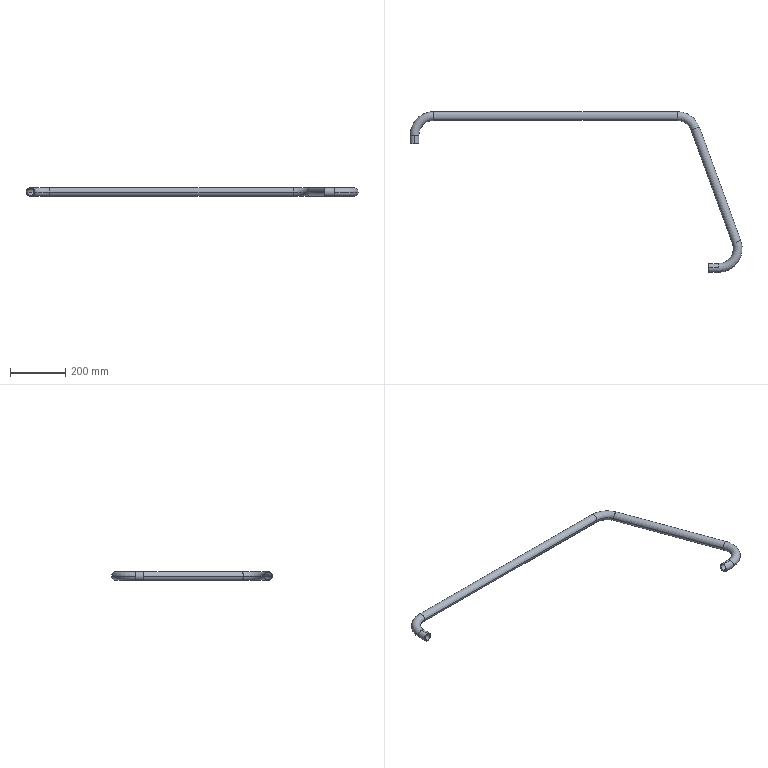Part | SolidWorks | features Sweep 1 | 1 solid | 30 faces | box 1202 x 582 x 32 mm | volume 468025 mm3 | cylinder 16 | torus 12 | plane 2 | commonest cylinder face diameters 26 x8 32 x8
STEP:
#1=CARTESIAN_POINT('',(1153.776,-360.505,0.));
#2=VERTEX_POINT('',#1);
#3=CARTESIAN_POINT('',(1178.208,-351.612,0.));
#4=VERTEX_POINT('',#3);
#5=CARTESIAN_POINT('',(1165.992,-356.059,0.));
#6=DIRECTION('',(-0.342,0.9397,0.));
#7=DIRECTION('',(0.,0.,1.));
#8=AXIS2_PLACEMENT_3D('',#5,#6,#7);
#9=CIRCLE('',#8,13.);
#10=EDGE_CURVE('',#2,#4,#9,.T.);
#11=ORIENTED_EDGE('',*,*,#10,.T.);
#12=CARTESIAN_POINT('',(1100.213,-463.,0.));
#13=VERTEX_POINT('',#12);
#14=CARTESIAN_POINT('',(1100.213,-380.,0.));
#15=DIRECTION('',(0.,0.,-1.));
#16=DIRECTION('',(-1.,0.,0.));
#17=AXIS2_PLACEMENT_3D('',#14,#15,#16);
#18=CIRCLE('',#17,83.);
#19=EDGE_CURVE('',#4,#13,#18,.T.);
#20=ORIENTED_EDGE('',*,*,#19,.T.);
#21=CARTESIAN_POINT('',(1100.213,-450.,13.));
#22=VERTEX_POINT('',#21);
#23=CARTESIAN_POINT('',(1100.213,-450.,0.));
#24=DIRECTION('',(1.,0.,0.));
#25=DIRECTION('',(0.,0.,1.));
#26=AXIS2_PLACEMENT_3D('',#23,#24,#25);
#27=CIRCLE('',#26,13.);
#28=EDGE_CURVE('',#22,#13,#27,.T.);
#29=ORIENTED_EDGE('',*,*,#28,.F.);
#30=CARTESIAN_POINT('',(1100.213,-437.,0.));
#31=VERTEX_POINT('',#30);
#32=CARTESIAN_POINT('',(1100.213,-450.,0.));
#33=DIRECTION('',(1.,0.,0.));
#34=DIRECTION('',(0.,0.,1.));
#35=AXIS2_PLACEMENT_3D('',#32,#33,#34);
#36=CIRCLE('',#35,13.);
#37=EDGE_CURVE('',#31,#22,#36,.T.);
#38=ORIENTED_EDGE('',*,*,#37,.F.);
#39=CARTESIAN_POINT('',(1100.213,-380.,0.));
#40=DIRECTION('',(0.,0.,-1.));
#41=DIRECTION('',(-1.,0.,0.));
#42=AXIS2_PLACEMENT_3D('',#39,#40,#41);
#43=CIRCLE('',#42,57.);
#44=EDGE_CURVE('',#2,#31,#43,.T.);
#45=ORIENTED_EDGE('',*,*,#44,.F.);
#46=EDGE_LOOP('',(#11,#20,#29,#38,#45));
#47=FACE_OUTER_BOUND('',#46,.T.);
#48=CARTESIAN_POINT('',(1100.213,-380.,0.));
#49=DIRECTION('',(0.,0.,-1.));
#50=DIRECTION('',(-1.,0.,0.));
#51=AXIS2_PLACEMENT_3D('',#48,#49,#50);
#52=TOROIDAL_SURFACE('',#51,70.,13.);
#53=ADVANCED_FACE('',(#47),#52,.F.);
#54=CARTESIAN_POINT('',(950.985,87.,0.));
#55=VERTEX_POINT('',#54);
#56=CARTESIAN_POINT('',(950.985,113.,0.));
#57=VERTEX_POINT('',#56);
#58=CARTESIAN_POINT('',(950.985,100.,0.));
#59=DIRECTION('',(-1.,0.,0.));
#60=DIRECTION('',(0.,0.,1.));
#61=AXIS2_PLACEMENT_3D('',#58,#59,#60);
#62=CIRCLE('',#61,13.);
#63=EDGE_CURVE('',#55,#57,#62,.T.);
#64=ORIENTED_EDGE('',*,*,#63,.T.);
#65=CARTESIAN_POINT('',(1028.98,58.388,0.));
#66=VERTEX_POINT('',#65);
#67=CARTESIAN_POINT('',(950.985,30.,0.));
#68=DIRECTION('',(0.,0.,-1.));
#69=DIRECTION('',(-1.,0.,0.));
#70=AXIS2_PLACEMENT_3D('',#67,#68,#69);
#71=CIRCLE('',#70,83.);
#72=EDGE_CURVE('',#57,#66,#71,.T.);
#73=ORIENTED_EDGE('',*,*,#72,.T.);
#74=CARTESIAN_POINT('',(1004.548,49.495,0.));
#75=VERTEX_POINT('',#74);
#76=CARTESIAN_POINT('',(1016.764,53.941,0.));
#77=DIRECTION('',(-0.342,0.9397,0.));
#78=DIRECTION('',(0.,0.,1.));
#79=AXIS2_PLACEMENT_3D('',#76,#77,#78);
#80=CIRCLE('',#79,13.);
#81=EDGE_CURVE('',#75,#66,#80,.T.);
#82=ORIENTED_EDGE('',*,*,#81,.F.);
#83=CARTESIAN_POINT('',(950.985,30.,0.));
#84=DIRECTION('',(0.,0.,-1.));
#85=DIRECTION('',(-1.,0.,0.));
#86=AXIS2_PLACEMENT_3D('',#83,#84,#85);
#87=CIRCLE('',#86,57.);
#88=EDGE_CURVE('',#55,#75,#87,.T.);
#89=ORIENTED_EDGE('',*,*,#88,.F.);
#90=EDGE_LOOP('',(#64,#73,#82,#89));
#91=FACE_OUTER_BOUND('',#90,.T.);
#92=CARTESIAN_POINT('',(950.985,30.,0.));
#93=DIRECTION('',(0.,0.,-1.));
#94=DIRECTION('',(-1.,0.,0.));
#95=AXIS2_PLACEMENT_3D('',#92,#93,#94);
#96=TOROIDAL_SURFACE('',#95,70.,13.);
#97=ADVANCED_FACE('',(#91),#96,.F.);
#98=CARTESIAN_POINT('',(0.,30.,13.));
#99=VERTEX_POINT('',#98);
#100=CARTESIAN_POINT('',(-13.,30.,0.));
#101=VERTEX_POINT('',#100);
#102=CARTESIAN_POINT('',(0.,30.,0.));
#103=DIRECTION('',(0.,-1.,0.));
#104=DIRECTION('',(0.,0.,1.));
#105=AXIS2_PLACEMENT_3D('',#102,#103,#104);
#106=CIRCLE('',#105,13.);
#107=EDGE_CURVE('',#99,#101,#106,.T.);
#108=ORIENTED_EDGE('',*,*,#107,.T.);
#109=CARTESIAN_POINT('',(70.,113.,0.));
#110=VERTEX_POINT('',#109);
#111=CARTESIAN_POINT('',(70.,30.,0.));
#112=DIRECTION('',(0.,0.,-1.));
#113=DIRECTION('',(-1.,0.,0.));
#114=AXIS2_PLACEMENT_3D('',#111,#112,#113);
#115=CIRCLE('',#114,83.);
#116=EDGE_CURVE('',#101,#110,#115,.T.);
#117=ORIENTED_EDGE('',*,*,#116,.T.);
#118=CARTESIAN_POINT('',(70.,87.,0.));
#119=VERTEX_POINT('',#118);
#120=CARTESIAN_POINT('',(70.,100.,0.));
#121=DIRECTION('',(-1.,0.,0.));
#122=DIRECTION('',(0.,0.,1.));
#123=AXIS2_PLACEMENT_3D('',#120,#121,#122);
#124=CIRCLE('',#123,13.);
#125=EDGE_CURVE('',#119,#110,#124,.T.);
#126=ORIENTED_EDGE('',*,*,#125,.F.);
#127=CARTESIAN_POINT('',(13.,30.,0.));
#128=VERTEX_POINT('',#127);
#129=CARTESIAN_POINT('',(70.,30.,0.));
#130=DIRECTION('',(0.,0.,-1.));
#131=DIRECTION('',(-1.,0.,0.));
#132=AXIS2_PLACEMENT_3D('',#129,#130,#131);
#133=CIRCLE('',#132,57.);
#134=EDGE_CURVE('',#128,#119,#133,.T.);
#135=ORIENTED_EDGE('',*,*,#134,.F.);
#136=CARTESIAN_POINT('',(0.,30.,0.));
#137=DIRECTION('',(0.,-1.,0.));
#138=DIRECTION('',(0.,0.,1.));
#139=AXIS2_PLACEMENT_3D('',#136,#137,#138);
#140=CIRCLE('',#139,13.);
#141=EDGE_CURVE('',#128,#99,#140,.T.);
#142=ORIENTED_EDGE('',*,*,#141,.T.);
#143=EDGE_LOOP('',(#108,#117,#126,#135,#142));
#144=FACE_OUTER_BOUND('',#143,.T.);
#145=CARTESIAN_POINT('',(70.,30.,0.));
#146=DIRECTION('',(0.,0.,-1.));
#147=DIRECTION('',(-1.,0.,0.));
#148=AXIS2_PLACEMENT_3D('',#145,#146,#147);
#149=TOROIDAL_SURFACE('',#148,70.,13.);
#150=ADVANCED_FACE('',(#144),#149,.F.);
#151=CARTESIAN_POINT('',(1150.957,-361.531,0.));
#152=VERTEX_POINT('',#151);
#153=CARTESIAN_POINT('',(1181.027,-350.586,0.));
#154=VERTEX_POINT('',#153);
#155=CARTESIAN_POINT('',(1165.992,-356.059,0.));
#156=DIRECTION('',(0.342,-0.9397,0.));
#157=DIRECTION('',(0.,0.,1.));
#158=AXIS2_PLACEMENT_3D('',#155,#156,#157);
#159=CIRCLE('',#158,16.);
#160=EDGE_CURVE('',#152,#154,#159,.T.);
#161=ORIENTED_EDGE('',*,*,#160,.T.);
#162=CARTESIAN_POINT('',(1100.213,-466.,0.));
#163=VERTEX_POINT('',#162);
#164=CARTESIAN_POINT('',(1100.213,-380.,0.));
#165=DIRECTION('',(0.,0.,-1.));
#166=DIRECTION('',(-1.,0.,0.));
#167=AXIS2_PLACEMENT_3D('',#164,#165,#166);
#168=CIRCLE('',#167,86.);
#169=EDGE_CURVE('',#154,#163,#168,.T.);
#170=ORIENTED_EDGE('',*,*,#169,.T.);
#171=CARTESIAN_POINT('',(1100.213,-450.,-16.));
#172=VERTEX_POINT('',#171);
#173=CARTESIAN_POINT('',(1100.213,-450.,0.));
#174=DIRECTION('',(-1.,0.,0.));
#175=DIRECTION('',(0.,0.,1.));
#176=AXIS2_PLACEMENT_3D('',#173,#174,#175);
#177=CIRCLE('',#176,16.);
#178=EDGE_CURVE('',#172,#163,#177,.T.);
#179=ORIENTED_EDGE('',*,*,#178,.F.);
#180=CARTESIAN_POINT('',(1100.213,-434.,0.));
#181=VERTEX_POINT('',#180);
#182=CARTESIAN_POINT('',(1100.213,-450.,0.));
#183=DIRECTION('',(-1.,0.,0.));
#184=DIRECTION('',(0.,0.,1.));
#185=AXIS2_PLACEMENT_3D('',#182,#183,#184);
#186=CIRCLE('',#185,16.);
#187=EDGE_CURVE('',#181,#172,#186,.T.);
#188=ORIENTED_EDGE('',*,*,#187,.F.);
#189=CARTESIAN_POINT('',(1100.213,-380.,0.));
#190=DIRECTION('',(0.,0.,-1.));
#191=DIRECTION('',(-1.,0.,0.));
#192=AXIS2_PLACEMENT_3D('',#189,#190,#191);
#193=CIRCLE('',#192,54.);
#194=EDGE_CURVE('',#152,#181,#193,.T.);
#195=ORIENTED_EDGE('',*,*,#194,.F.);
#196=EDGE_LOOP('',(#161,#170,#179,#188,#195));
#197=FACE_OUTER_BOUND('',#196,.T.);
#198=CARTESIAN_POINT('',(1100.213,-380.,0.));
#199=DIRECTION('',(0.,0.,-1.));
#200=DIRECTION('',(-1.,0.,0.));
#201=AXIS2_PLACEMENT_3D('',#198,#199,#200);
#202=TOROIDAL_SURFACE('',#201,70.,16.);
#203=ADVANCED_FACE('',(#197),#202,.T.);
#204=CARTESIAN_POINT('',(950.985,84.,0.));
#205=VERTEX_POINT('',#204);
#206=CARTESIAN_POINT('',(950.985,116.,0.));
#207=VERTEX_POINT('',#206);
#208=CARTESIAN_POINT('',(950.985,100.,0.));
#209=DIRECTION('',(1.,0.,0.));
#210=DIRECTION('',(0.,0.,1.));
#211=AXIS2_PLACEMENT_3D('',#208,#209,#210);
#212=CIRCLE('',#211,16.);
#213=EDGE_CURVE('',#205,#207,#212,.T.);
#214=ORIENTED_EDGE('',*,*,#213,.T.);
#215=CARTESIAN_POINT('',(1031.799,59.414,0.));
#216=VERTEX_POINT('',#215);
#217=CARTESIAN_POINT('',(950.985,30.,0.));
#218=DIRECTION('',(0.,0.,-1.));
#219=DIRECTION('',(-1.,0.,0.));
#220=AXIS2_PLACEMENT_3D('',#217,#218,#219);
#221=CIRCLE('',#220,86.);
#222=EDGE_CURVE('',#207,#216,#221,.T.);
#223=ORIENTED_EDGE('',*,*,#222,.T.);
#224=CARTESIAN_POINT('',(1001.729,48.469,0.));
#225=VERTEX_POINT('',#224);
#226=CARTESIAN_POINT('',(1016.764,53.941,0.));
#227=DIRECTION('',(0.342,-0.9397,0.));
#228=DIRECTION('',(0.,0.,1.));
#229=AXIS2_PLACEMENT_3D('',#226,#227,#228);
#230=CIRCLE('',#229,16.);
#231=EDGE_CURVE('',#225,#216,#230,.T.);
#232=ORIENTED_EDGE('',*,*,#231,.F.);
#233=CARTESIAN_POINT('',(950.985,30.,0.));
#234=DIRECTION('',(0.,0.,-1.));
#235=DIRECTION('',(-1.,0.,0.));
#236=AXIS2_PLACEMENT_3D('',#233,#234,#235);
#237=CIRCLE('',#236,54.);
#238=EDGE_CURVE('',#205,#225,#237,.T.);
#239=ORIENTED_EDGE('',*,*,#238,.F.);
#240=EDGE_LOOP('',(#214,#223,#232,#239));
#241=FACE_OUTER_BOUND('',#240,.T.);
#242=CARTESIAN_POINT('',(950.985,30.,0.));
#243=DIRECTION('',(0.,0.,-1.));
#244=DIRECTION('',(-1.,0.,0.));
#245=AXIS2_PLACEMENT_3D('',#242,#243,#244);
#246=TOROIDAL_SURFACE('',#245,70.,16.);
#247=ADVANCED_FACE('',(#241),#246,.T.);
#248=CARTESIAN_POINT('',(0.,30.,-16.));
#249=VERTEX_POINT('',#248);
#250=CARTESIAN_POINT('',(-16.,30.,0.));
#251=VERTEX_POINT('',#250);
#252=CARTESIAN_POINT('',(0.,30.,0.));
#253=DIRECTION('',(0.,1.,0.));
#254=DIRECTION('',(0.,0.,1.));
#255=AXIS2_PLACEMENT_3D('',#252,#253,#254);
#256=CIRCLE('',#255,16.);
#257=EDGE_CURVE('',#249,#251,#256,.T.);
#258=ORIENTED_EDGE('',*,*,#257,.T.);
#259=CARTESIAN_POINT('',(70.,116.,0.));
#260=VERTEX_POINT('',#259);
#261=CARTESIAN_POINT('',(70.,30.,0.));
#262=DIRECTION('',(0.,0.,-1.));
#263=DIRECTION('',(-1.,0.,0.));
#264=AXIS2_PLACEMENT_3D('',#261,#262,#263);
#265=CIRCLE('',#264,86.);
#266=EDGE_CURVE('',#251,#260,#265,.T.);
#267=ORIENTED_EDGE('',*,*,#266,.T.);
#268=CARTESIAN_POINT('',(70.,84.,0.));
#269=VERTEX_POINT('',#268);
#270=CARTESIAN_POINT('',(70.,100.,0.));
#271=DIRECTION('',(1.,0.,0.));
#272=DIRECTION('',(0.,0.,1.));
#273=AXIS2_PLACEMENT_3D('',#270,#271,#272);
#274=CIRCLE('',#273,16.);
#275=EDGE_CURVE('',#269,#260,#274,.T.);
#276=ORIENTED_EDGE('',*,*,#275,.F.);
#277=CARTESIAN_POINT('',(16.,30.,0.));
#278=VERTEX_POINT('',#277);
#279=CARTESIAN_POINT('',(70.,30.,0.));
#280=DIRECTION('',(0.,0.,-1.));
#281=DIRECTION('',(-1.,0.,0.));
#282=AXIS2_PLACEMENT_3D('',#279,#280,#281);
#283=CIRCLE('',#282,54.);
#284=EDGE_CURVE('',#278,#269,#283,.T.);
#285=ORIENTED_EDGE('',*,*,#284,.F.);
#286=CARTESIAN_POINT('',(0.,30.,0.));
#287=DIRECTION('',(0.,1.,0.));
#288=DIRECTION('',(0.,0.,1.));
#289=AXIS2_PLACEMENT_3D('',#286,#287,#288);
#290=CIRCLE('',#289,16.);
#291=EDGE_CURVE('',#278,#249,#290,.T.);
#292=ORIENTED_EDGE('',*,*,#291,.T.);
#293=EDGE_LOOP('',(#258,#267,#276,#285,#292));
#294=FACE_OUTER_BOUND('',#293,.T.);
#295=CARTESIAN_POINT('',(70.,30.,0.));
#296=DIRECTION('',(0.,0.,-1.));
#297=DIRECTION('',(-1.,0.,0.));
#298=AXIS2_PLACEMENT_3D('',#295,#296,#297);
#299=TOROIDAL_SURFACE('',#298,70.,16.);
#300=ADVANCED_FACE('',(#294),#299,.T.);
#301=ORIENTED_EDGE('',*,*,#28,.T.);
#302=CARTESIAN_POINT('',(1100.213,-450.,-13.));
#303=VERTEX_POINT('',#302);
#304=CARTESIAN_POINT('',(1100.213,-450.,0.));
#305=DIRECTION('',(1.,0.,0.));
#306=DIRECTION('',(0.,0.,1.));
#307=AXIS2_PLACEMENT_3D('',#304,#305,#306);
#308=CIRCLE('',#307,13.);
#309=EDGE_CURVE('',#13,#303,#308,.T.);
#310=ORIENTED_EDGE('',*,*,#309,.T.);
#311=CARTESIAN_POINT('',(1065.,-450.,-13.));
#312=VERTEX_POINT('',#311);
#313=CARTESIAN_POINT('',(1100.213,-450.,-13.));
#314=DIRECTION('',(-1.,0.,0.));
#315=VECTOR('',#314,1000.);
#316=LINE('',#313,#315);
#317=EDGE_CURVE('',#303,#312,#316,.T.);
#318=ORIENTED_EDGE('',*,*,#317,.T.);
#319=CARTESIAN_POINT('',(1065.,-450.,13.));
#320=VERTEX_POINT('',#319);
#321=CARTESIAN_POINT('',(1065.,-450.,0.));
#322=DIRECTION('',(1.,0.,0.));
#323=DIRECTION('',(0.,0.,1.));
#324=AXIS2_PLACEMENT_3D('',#321,#322,#323);
#325=CIRCLE('',#324,13.);
#326=EDGE_CURVE('',#320,#312,#325,.T.);
#327=ORIENTED_EDGE('',*,*,#326,.F.);
#328=CARTESIAN_POINT('',(1100.213,-450.,13.));
#329=DIRECTION('',(-1.,0.,0.));
#330=VECTOR('',#329,1000.);
#331=LINE('',#328,#330);
#332=EDGE_CURVE('',#22,#320,#331,.T.);
#333=ORIENTED_EDGE('',*,*,#332,.F.);
#334=EDGE_LOOP('',(#301,#310,#318,#327,#333));
#335=FACE_OUTER_BOUND('',#334,.T.);
#336=CARTESIAN_POINT('',(1100.213,-450.,0.));
#337=DIRECTION('',(-1.,0.,0.));
#338=DIRECTION('',(0.,0.,1.));
#339=AXIS2_PLACEMENT_3D('',#336,#337,#338);
#340=CYLINDRICAL_SURFACE('',#339,13.);
#341=ADVANCED_FACE('',(#335),#340,.F.);
#342=CARTESIAN_POINT('',(1016.764,53.941,0.));
#343=DIRECTION('',(-0.342,0.9397,0.));
#344=DIRECTION('',(0.,0.,1.));
#345=AXIS2_PLACEMENT_3D('',#342,#343,#344);
#346=CIRCLE('',#345,13.);
#347=EDGE_CURVE('',#66,#75,#346,.T.);
#348=ORIENTED_EDGE('',*,*,#347,.T.);
#349=CARTESIAN_POINT('',(1004.548,49.495,0.));
#350=DIRECTION('',(0.342,-0.9397,0.));
#351=VECTOR('',#350,1000.);
#352=LINE('',#349,#351);
#353=EDGE_CURVE('',#75,#2,#352,.T.);
#354=ORIENTED_EDGE('',*,*,#353,.T.);
#355=CARTESIAN_POINT('',(1165.992,-356.059,0.));
#356=DIRECTION('',(-0.342,0.9397,0.));
#357=DIRECTION('',(0.,0.,1.));
#358=AXIS2_PLACEMENT_3D('',#355,#356,#357);
#359=CIRCLE('',#358,13.);
#360=EDGE_CURVE('',#4,#2,#359,.T.);
#361=ORIENTED_EDGE('',*,*,#360,.F.);
#362=CARTESIAN_POINT('',(1028.98,58.388,0.));
#363=DIRECTION('',(0.342,-0.9397,0.));
#364=VECTOR('',#363,1000.);
#365=LINE('',#362,#364);
#366=EDGE_CURVE('',#66,#4,#365,.T.);
#367=ORIENTED_EDGE('',*,*,#366,.F.);
#368=EDGE_LOOP('',(#348,#354,#361,#367));
#369=FACE_OUTER_BOUND('',#368,.T.);
#370=CARTESIAN_POINT('',(1016.764,53.941,0.));
#371=DIRECTION('',(0.342,-0.9397,0.));
#372=DIRECTION('',(0.9397,0.342,0.));
#373=AXIS2_PLACEMENT_3D('',#370,#371,#372);
#374=CYLINDRICAL_SURFACE('',#373,13.);
#375=ADVANCED_FACE('',(#369),#374,.F.);
#376=CARTESIAN_POINT('',(70.,100.,0.));
#377=DIRECTION('',(-1.,0.,0.));
#378=DIRECTION('',(0.,0.,1.));
#379=AXIS2_PLACEMENT_3D('',#376,#377,#378);
#380=CIRCLE('',#379,13.);
#381=EDGE_CURVE('',#110,#119,#380,.T.);
#382=ORIENTED_EDGE('',*,*,#381,.T.);
#383=CARTESIAN_POINT('',(70.,87.,0.));
#384=DIRECTION('',(1.,0.,0.));
#385=VECTOR('',#384,1000.);
#386=LINE('',#383,#385);
#387=EDGE_CURVE('',#119,#55,#386,.T.);
#388=ORIENTED_EDGE('',*,*,#387,.T.);
#389=CARTESIAN_POINT('',(950.985,100.,0.));
#390=DIRECTION('',(-1.,0.,0.));
#391=DIRECTION('',(0.,0.,1.));
#392=AXIS2_PLACEMENT_3D('',#389,#390,#391);
#393=CIRCLE('',#392,13.);
#394=EDGE_CURVE('',#57,#55,#393,.T.);
#395=ORIENTED_EDGE('',*,*,#394,.F.);
#396=CARTESIAN_POINT('',(70.,113.,0.));
#397=DIRECTION('',(1.,0.,0.));
#398=VECTOR('',#397,1000.);
#399=LINE('',#396,#398);
#400=EDGE_CURVE('',#110,#57,#399,.T.);
#401=ORIENTED_EDGE('',*,*,#400,.F.);
#402=EDGE_LOOP('',(#382,#388,#395,#401));
#403=FACE_OUTER_BOUND('',#402,.T.);
#404=CARTESIAN_POINT('',(70.,100.,0.));
#405=DIRECTION('',(1.,0.,0.));
#406=DIRECTION('',(0.,1.,0.));
#407=AXIS2_PLACEMENT_3D('',#404,#405,#406);
#408=CYLINDRICAL_SURFACE('',#407,13.);
#409=ADVANCED_FACE('',(#403),#408,.F.);
#410=CARTESIAN_POINT('',(0.,0.,13.));
#411=VERTEX_POINT('',#410);
#412=CARTESIAN_POINT('',(0.,0.,-13.));
#413=VERTEX_POINT('',#412);
#414=CARTESIAN_POINT('',(0.,0.,0.));
#415=DIRECTION('',(0.,-1.,0.));
#416=DIRECTION('',(0.,0.,1.));
#417=AXIS2_PLACEMENT_3D('',#414,#415,#416);
#418=CIRCLE('',#417,13.);
#419=EDGE_CURVE('',#411,#413,#418,.T.);
#420=ORIENTED_EDGE('',*,*,#419,.T.);
#421=CARTESIAN_POINT('',(0.,30.,-13.));
#422=VERTEX_POINT('',#421);
#423=CARTESIAN_POINT('',(0.,0.,-13.));
#424=DIRECTION('',(0.,1.,0.));
#425=VECTOR('',#424,1000.);
#426=LINE('',#423,#425);
#427=EDGE_CURVE('',#413,#422,#426,.T.);
#428=ORIENTED_EDGE('',*,*,#427,.T.);
#429=CARTESIAN_POINT('',(0.,30.,0.));
#430=DIRECTION('',(0.,-1.,0.));
#431=DIRECTION('',(0.,0.,1.));
#432=AXIS2_PLACEMENT_3D('',#429,#430,#431);
#433=CIRCLE('',#432,13.);
#434=EDGE_CURVE('',#101,#422,#433,.T.);
#435=ORIENTED_EDGE('',*,*,#434,.F.);
#436=ORIENTED_EDGE('',*,*,#107,.F.);
#437=CARTESIAN_POINT('',(0.,0.,13.));
#438=DIRECTION('',(0.,1.,0.));
#439=VECTOR('',#438,1000.);
#440=LINE('',#437,#439);
#441=EDGE_CURVE('',#411,#99,#440,.T.);
#442=ORIENTED_EDGE('',*,*,#441,.F.);
#443=EDGE_LOOP('',(#420,#428,#435,#436,#442));
#444=FACE_OUTER_BOUND('',#443,.T.);
#445=CARTESIAN_POINT('',(0.,0.,0.));
#446=DIRECTION('',(0.,1.,0.));
#447=DIRECTION('',(0.,0.,1.));
#448=AXIS2_PLACEMENT_3D('',#445,#446,#447);
#449=CYLINDRICAL_SURFACE('',#448,13.);
#450=ADVANCED_FACE('',(#444),#449,.F.);
#451=CARTESIAN_POINT('',(1100.213,-450.,16.));
#452=VERTEX_POINT('',#451);
#453=CARTESIAN_POINT('',(1100.213,-450.,0.));
#454=DIRECTION('',(-1.,0.,0.));
#455=DIRECTION('',(0.,0.,1.));
#456=AXIS2_PLACEMENT_3D('',#453,#454,#455);
#457=CIRCLE('',#456,16.);
#458=EDGE_CURVE('',#452,#181,#457,.T.);
#459=ORIENTED_EDGE('',*,*,#458,.T.);
#460=ORIENTED_EDGE('',*,*,#187,.T.);
#461=CARTESIAN_POINT('',(1065.,-450.,-16.));
#462=VERTEX_POINT('',#461);
#463=CARTESIAN_POINT('',(1100.213,-450.,-16.));
#464=DIRECTION('',(-1.,0.,0.));
#465=VECTOR('',#464,1000.);
#466=LINE('',#463,#465);
#467=EDGE_CURVE('',#172,#462,#466,.T.);
#468=ORIENTED_EDGE('',*,*,#467,.T.);
#469=CARTESIAN_POINT('',(1065.,-450.,16.));
#470=VERTEX_POINT('',#469);
#471=CARTESIAN_POINT('',(1065.,-450.,0.));
#472=DIRECTION('',(-1.,0.,0.));
#473=DIRECTION('',(0.,0.,1.));
#474=AXIS2_PLACEMENT_3D('',#471,#472,#473);
#475=CIRCLE('',#474,16.);
#476=EDGE_CURVE('',#470,#462,#475,.T.);
#477=ORIENTED_EDGE('',*,*,#476,.F.);
#478=CARTESIAN_POINT('',(1100.213,-450.,16.));
#479=DIRECTION('',(-1.,0.,0.));
#480=VECTOR('',#479,1000.);
#481=LINE('',#478,#480);
#482=EDGE_CURVE('',#452,#470,#481,.T.);
#483=ORIENTED_EDGE('',*,*,#482,.F.);
#484=EDGE_LOOP('',(#459,#460,#468,#477,#483));
#485=FACE_OUTER_BOUND('',#484,.T.);
#486=CARTESIAN_POINT('',(1100.213,-450.,0.));
#487=DIRECTION('',(-1.,0.,0.));
#488=DIRECTION('',(0.,0.,1.));
#489=AXIS2_PLACEMENT_3D('',#486,#487,#488);
#490=CYLINDRICAL_SURFACE('',#489,16.);
#491=ADVANCED_FACE('',(#485),#490,.T.);
#492=CARTESIAN_POINT('',(1016.764,53.941,0.));
#493=DIRECTION('',(0.342,-0.9397,0.));
#494=DIRECTION('',(0.,0.,1.));
#495=AXIS2_PLACEMENT_3D('',#492,#493,#494);
#496=CIRCLE('',#495,16.);
#497=EDGE_CURVE('',#216,#225,#496,.T.);
#498=ORIENTED_EDGE('',*,*,#497,.T.);
#499=CARTESIAN_POINT('',(1001.729,48.469,0.));
#500=DIRECTION('',(0.342,-0.9397,0.));
#501=VECTOR('',#500,1000.);
#502=LINE('',#499,#501);
#503=EDGE_CURVE('',#225,#152,#502,.T.);
#504=ORIENTED_EDGE('',*,*,#503,.T.);
#505=CARTESIAN_POINT('',(1165.992,-356.059,0.));
#506=DIRECTION('',(0.342,-0.9397,0.));
#507=DIRECTION('',(0.,0.,1.));
#508=AXIS2_PLACEMENT_3D('',#505,#506,#507);
#509=CIRCLE('',#508,16.);
#510=EDGE_CURVE('',#154,#152,#509,.T.);
#511=ORIENTED_EDGE('',*,*,#510,.F.);
#512=CARTESIAN_POINT('',(1031.799,59.414,0.));
#513=DIRECTION('',(0.342,-0.9397,0.));
#514=VECTOR('',#513,1000.);
#515=LINE('',#512,#514);
#516=EDGE_CURVE('',#216,#154,#515,.T.);
#517=ORIENTED_EDGE('',*,*,#516,.F.);
#518=EDGE_LOOP('',(#498,#504,#511,#517));
#519=FACE_OUTER_BOUND('',#518,.T.);
#520=CARTESIAN_POINT('',(1016.764,53.941,0.));
#521=DIRECTION('',(0.342,-0.9397,0.));
#522=DIRECTION('',(0.9397,0.342,0.));
#523=AXIS2_PLACEMENT_3D('',#520,#521,#522);
#524=CYLINDRICAL_SURFACE('',#523,16.);
#525=ADVANCED_FACE('',(#519),#524,.T.);
#526=CARTESIAN_POINT('',(70.,100.,0.));
#527=DIRECTION('',(1.,0.,0.));
#528=DIRECTION('',(0.,0.,1.));
#529=AXIS2_PLACEMENT_3D('',#526,#527,#528);
#530=CIRCLE('',#529,16.);
#531=EDGE_CURVE('',#260,#269,#530,.T.);
#532=ORIENTED_EDGE('',*,*,#531,.T.);
#533=CARTESIAN_POINT('',(70.,84.,0.));
#534=DIRECTION('',(1.,0.,0.));
#535=VECTOR('',#534,1000.);
#536=LINE('',#533,#535);
#537=EDGE_CURVE('',#269,#205,#536,.T.);
#538=ORIENTED_EDGE('',*,*,#537,.T.);
#539=CARTESIAN_POINT('',(950.985,100.,0.));
#540=DIRECTION('',(1.,0.,0.));
#541=DIRECTION('',(0.,0.,1.));
#542=AXIS2_PLACEMENT_3D('',#539,#540,#541);
#543=CIRCLE('',#542,16.);
#544=EDGE_CURVE('',#207,#205,#543,.T.);
#545=ORIENTED_EDGE('',*,*,#544,.F.);
#546=CARTESIAN_POINT('',(70.,116.,0.));
#547=DIRECTION('',(1.,0.,0.));
#548=VECTOR('',#547,1000.);
#549=LINE('',#546,#548);
#550=EDGE_CURVE('',#260,#207,#549,.T.);
#551=ORIENTED_EDGE('',*,*,#550,.F.);
#552=EDGE_LOOP('',(#532,#538,#545,#551));
#553=FACE_OUTER_BOUND('',#552,.T.);
#554=CARTESIAN_POINT('',(70.,100.,0.));
#555=DIRECTION('',(1.,0.,0.));
#556=DIRECTION('',(0.,1.,0.));
#557=AXIS2_PLACEMENT_3D('',#554,#555,#556);
#558=CYLINDRICAL_SURFACE('',#557,16.);
#559=ADVANCED_FACE('',(#553),#558,.T.);
#560=CARTESIAN_POINT('',(0.,0.,16.));
#561=VERTEX_POINT('',#560);
#562=CARTESIAN_POINT('',(0.,0.,-16.));
#563=VERTEX_POINT('',#562);
#564=CARTESIAN_POINT('',(0.,0.,0.));
#565=DIRECTION('',(0.,1.,0.));
#566=DIRECTION('',(0.,0.,1.));
#567=AXIS2_PLACEMENT_3D('',#564,#565,#566);
#568=CIRCLE('',#567,16.);
#569=EDGE_CURVE('',#561,#563,#568,.T.);
#570=ORIENTED_EDGE('',*,*,#569,.T.);
#571=CARTESIAN_POINT('',(0.,0.,-16.));
#572=DIRECTION('',(0.,1.,0.));
#573=VECTOR('',#572,1000.);
#574=LINE('',#571,#573);
#575=EDGE_CURVE('',#563,#249,#574,.T.);
#576=ORIENTED_EDGE('',*,*,#575,.T.);
#577=ORIENTED_EDGE('',*,*,#291,.F.);
#578=CARTESIAN_POINT('',(0.,30.,16.));
#579=VERTEX_POINT('',#578);
#580=CARTESIAN_POINT('',(0.,30.,0.));
#581=DIRECTION('',(0.,1.,0.));
#582=DIRECTION('',(0.,0.,1.));
#583=AXIS2_PLACEMENT_3D('',#580,#581,#582);
#584=CIRCLE('',#583,16.);
#585=EDGE_CURVE('',#579,#278,#584,.T.);
#586=ORIENTED_EDGE('',*,*,#585,.F.);
#587=CARTESIAN_POINT('',(0.,0.,16.));
#588=DIRECTION('',(0.,1.,0.));
#589=VECTOR('',#588,1000.);
#590=LINE('',#587,#589);
#591=EDGE_CURVE('',#561,#579,#590,.T.);
#592=ORIENTED_EDGE('',*,*,#591,.F.);
#593=EDGE_LOOP('',(#570,#576,#577,#586,#592));
#594=FACE_OUTER_BOUND('',#593,.T.);
#595=CARTESIAN_POINT('',(0.,0.,0.));
#596=DIRECTION('',(0.,1.,0.));
#597=DIRECTION('',(0.,0.,1.));
#598=AXIS2_PLACEMENT_3D('',#595,#596,#597);
#599=CYLINDRICAL_SURFACE('',#598,16.);
#600=ADVANCED_FACE('',(#594),#599,.T.);
#601=ORIENTED_EDGE('',*,*,#317,.F.);
#602=CARTESIAN_POINT('',(1100.213,-450.,0.));
#603=DIRECTION('',(1.,0.,0.));
#604=DIRECTION('',(0.,0.,1.));
#605=AXIS2_PLACEMENT_3D('',#602,#603,#604);
#606=CIRCLE('',#605,13.);
#607=EDGE_CURVE('',#303,#31,#606,.T.);
#608=ORIENTED_EDGE('',*,*,#607,.T.);
#609=ORIENTED_EDGE('',*,*,#37,.T.);
#610=ORIENTED_EDGE('',*,*,#332,.T.);
#611=CARTESIAN_POINT('',(1065.,-450.,0.));
#612=DIRECTION('',(1.,0.,0.));
#613=DIRECTION('',(0.,0.,1.));
#614=AXIS2_PLACEMENT_3D('',#611,#612,#613);
#615=CIRCLE('',#614,13.);
#616=EDGE_CURVE('',#312,#320,#615,.T.);
#617=ORIENTED_EDGE('',*,*,#616,.F.);
#618=EDGE_LOOP('',(#601,#608,#609,#610,#617));
#619=FACE_OUTER_BOUND('',#618,.T.);
#620=CARTESIAN_POINT('',(1100.213,-450.,0.));
#621=DIRECTION('',(-1.,0.,0.));
#622=DIRECTION('',(0.,0.,1.));
#623=AXIS2_PLACEMENT_3D('',#620,#621,#622);
#624=CYLINDRICAL_SURFACE('',#623,13.);
#625=ADVANCED_FACE('',(#619),#624,.F.);
#626=ORIENTED_EDGE('',*,*,#19,.F.);
#627=ORIENTED_EDGE('',*,*,#360,.T.);
#628=ORIENTED_EDGE('',*,*,#44,.T.);
#629=ORIENTED_EDGE('',*,*,#607,.F.);
#630=ORIENTED_EDGE('',*,*,#309,.F.);
#631=EDGE_LOOP('',(#626,#627,#628,#629,#630));
#632=FACE_OUTER_BOUND('',#631,.T.);
#633=CARTESIAN_POINT('',(1100.213,-380.,0.));
#634=DIRECTION('',(0.,0.,-1.));
#635=DIRECTION('',(-1.,0.,0.));
#636=AXIS2_PLACEMENT_3D('',#633,#634,#635);
#637=TOROIDAL_SURFACE('',#636,70.,13.);
#638=ADVANCED_FACE('',(#632),#637,.F.);
#639=ORIENTED_EDGE('',*,*,#353,.F.);
#640=ORIENTED_EDGE('',*,*,#81,.T.);
#641=ORIENTED_EDGE('',*,*,#366,.T.);
#642=ORIENTED_EDGE('',*,*,#10,.F.);
#643=EDGE_LOOP('',(#639,#640,#641,#642));
#644=FACE_OUTER_BOUND('',#643,.T.);
#645=CARTESIAN_POINT('',(1016.764,53.941,0.));
#646=DIRECTION('',(0.342,-0.9397,0.));
#647=DIRECTION('',(0.9397,0.342,0.));
#648=AXIS2_PLACEMENT_3D('',#645,#646,#647);
#649=CYLINDRICAL_SURFACE('',#648,13.);
#650=ADVANCED_FACE('',(#644),#649,.F.);
#651=ORIENTED_EDGE('',*,*,#72,.F.);
#652=ORIENTED_EDGE('',*,*,#394,.T.);
#653=ORIENTED_EDGE('',*,*,#88,.T.);
#654=ORIENTED_EDGE('',*,*,#347,.F.);
#655=EDGE_LOOP('',(#651,#652,#653,#654));
#656=FACE_OUTER_BOUND('',#655,.T.);
#657=CARTESIAN_POINT('',(950.985,30.,0.));
#658=DIRECTION('',(0.,0.,-1.));
#659=DIRECTION('',(-1.,0.,0.));
#660=AXIS2_PLACEMENT_3D('',#657,#658,#659);
#661=TOROIDAL_SURFACE('',#660,70.,13.);
#662=ADVANCED_FACE('',(#656),#661,.F.);
#663=ORIENTED_EDGE('',*,*,#387,.F.);
#664=ORIENTED_EDGE('',*,*,#125,.T.);
#665=ORIENTED_EDGE('',*,*,#400,.T.);
#666=ORIENTED_EDGE('',*,*,#63,.F.);
#667=EDGE_LOOP('',(#663,#664,#665,#666));
#668=FACE_OUTER_BOUND('',#667,.T.);
#669=CARTESIAN_POINT('',(70.,100.,0.));
#670=DIRECTION('',(1.,0.,0.));
#671=DIRECTION('',(0.,1.,0.));
#672=AXIS2_PLACEMENT_3D('',#669,#670,#671);
#673=CYLINDRICAL_SURFACE('',#672,13.);
#674=ADVANCED_FACE('',(#668),#673,.F.);
#675=ORIENTED_EDGE('',*,*,#116,.F.);
#676=ORIENTED_EDGE('',*,*,#434,.T.);
#677=CARTESIAN_POINT('',(0.,30.,0.));
#678=DIRECTION('',(0.,-1.,0.));
#679=DIRECTION('',(0.,0.,1.));
#680=AXIS2_PLACEMENT_3D('',#677,#678,#679);
#681=CIRCLE('',#680,13.);
#682=EDGE_CURVE('',#422,#128,#681,.T.);
#683=ORIENTED_EDGE('',*,*,#682,.T.);
#684=ORIENTED_EDGE('',*,*,#134,.T.);
#685=ORIENTED_EDGE('',*,*,#381,.F.);
#686=EDGE_LOOP('',(#675,#676,#683,#684,#685));
#687=FACE_OUTER_BOUND('',#686,.T.);
#688=CARTESIAN_POINT('',(70.,30.,0.));
#689=DIRECTION('',(0.,0.,-1.));
#690=DIRECTION('',(-1.,0.,0.));
#691=AXIS2_PLACEMENT_3D('',#688,#689,#690);
#692=TOROIDAL_SURFACE('',#691,70.,13.);
#693=ADVANCED_FACE('',(#687),#692,.F.);
#694=ORIENTED_EDGE('',*,*,#427,.F.);
#695=CARTESIAN_POINT('',(0.,0.,0.));
#696=DIRECTION('',(0.,-1.,0.));
#697=DIRECTION('',(0.,0.,1.));
#698=AXIS2_PLACEMENT_3D('',#695,#696,#697);
#699=CIRCLE('',#698,13.);
#700=EDGE_CURVE('',#413,#411,#699,.T.);
#701=ORIENTED_EDGE('',*,*,#700,.T.);
#702=ORIENTED_EDGE('',*,*,#441,.T.);
#703=ORIENTED_EDGE('',*,*,#141,.F.);
#704=ORIENTED_EDGE('',*,*,#682,.F.);
#705=EDGE_LOOP('',(#694,#701,#702,#703,#704));
#706=FACE_OUTER_BOUND('',#705,.T.);
#707=CARTESIAN_POINT('',(0.,0.,0.));
#708=DIRECTION('',(0.,1.,0.));
#709=DIRECTION('',(0.,0.,1.));
#710=AXIS2_PLACEMENT_3D('',#707,#708,#709);
#711=CYLINDRICAL_SURFACE('',#710,13.);
#712=ADVANCED_FACE('',(#706),#711,.F.);
#713=ORIENTED_EDGE('',*,*,#326,.T.);
#714=ORIENTED_EDGE('',*,*,#616,.T.);
#715=EDGE_LOOP('',(#713,#714));
#716=FACE_BOUND('',#715,.T.);
#717=ORIENTED_EDGE('',*,*,#476,.T.);
#718=CARTESIAN_POINT('',(1065.,-450.,0.));
#719=DIRECTION('',(-1.,0.,0.));
#720=DIRECTION('',(0.,0.,1.));
#721=AXIS2_PLACEMENT_3D('',#718,#719,#720);
#722=CIRCLE('',#721,16.);
#723=EDGE_CURVE('',#462,#470,#722,.T.);
#724=ORIENTED_EDGE('',*,*,#723,.T.);
#725=EDGE_LOOP('',(#717,#724));
#726=FACE_OUTER_BOUND('',#725,.T.);
#727=CARTESIAN_POINT('',(1065.,-450.,0.));
#728=DIRECTION('',(-1.,0.,0.));
#729=DIRECTION('',(0.,0.,1.));
#730=AXIS2_PLACEMENT_3D('',#727,#728,#729);
#731=PLANE('',#730);
#732=ADVANCED_FACE('',(#716,#726),#731,.T.);
#733=ORIENTED_EDGE('',*,*,#419,.F.);
#734=ORIENTED_EDGE('',*,*,#700,.F.);
#735=EDGE_LOOP('',(#733,#734));
#736=FACE_BOUND('',#735,.T.);
#737=ORIENTED_EDGE('',*,*,#569,.F.);
#738=CARTESIAN_POINT('',(0.,0.,0.));
#739=DIRECTION('',(0.,1.,0.));
#740=DIRECTION('',(0.,0.,1.));
#741=AXIS2_PLACEMENT_3D('',#738,#739,#740);
#742=CIRCLE('',#741,16.);
#743=EDGE_CURVE('',#563,#561,#742,.T.);
#744=ORIENTED_EDGE('',*,*,#743,.F.);
#745=EDGE_LOOP('',(#737,#744));
#746=FACE_OUTER_BOUND('',#745,.T.);
#747=CARTESIAN_POINT('',(0.,0.,0.));
#748=DIRECTION('',(0.,1.,0.));
#749=DIRECTION('',(0.,0.,1.));
#750=AXIS2_PLACEMENT_3D('',#747,#748,#749);
#751=PLANE('',#750);
#752=ADVANCED_FACE('',(#736,#746),#751,.F.);
#753=ORIENTED_EDGE('',*,*,#467,.F.);
#754=ORIENTED_EDGE('',*,*,#178,.T.);
#755=CARTESIAN_POINT('',(1100.213,-450.,0.));
#756=DIRECTION('',(-1.,0.,0.));
#757=DIRECTION('',(0.,0.,1.));
#758=AXIS2_PLACEMENT_3D('',#755,#756,#757);
#759=CIRCLE('',#758,16.);
#760=EDGE_CURVE('',#163,#452,#759,.T.);
#761=ORIENTED_EDGE('',*,*,#760,.T.);
#762=ORIENTED_EDGE('',*,*,#482,.T.);
#763=ORIENTED_EDGE('',*,*,#723,.F.);
#764=EDGE_LOOP('',(#753,#754,#761,#762,#763));
#765=FACE_OUTER_BOUND('',#764,.T.);
#766=CARTESIAN_POINT('',(1100.213,-450.,0.));
#767=DIRECTION('',(-1.,0.,0.));
#768=DIRECTION('',(0.,0.,1.));
#769=AXIS2_PLACEMENT_3D('',#766,#767,#768);
#770=CYLINDRICAL_SURFACE('',#769,16.);
#771=ADVANCED_FACE('',(#765),#770,.T.);
#772=ORIENTED_EDGE('',*,*,#169,.F.);
#773=ORIENTED_EDGE('',*,*,#510,.T.);
#774=ORIENTED_EDGE('',*,*,#194,.T.);
#775=ORIENTED_EDGE('',*,*,#458,.F.);
#776=ORIENTED_EDGE('',*,*,#760,.F.);
#777=EDGE_LOOP('',(#772,#773,#774,#775,#776));
#778=FACE_OUTER_BOUND('',#777,.T.);
#779=CARTESIAN_POINT('',(1100.213,-380.,0.));
#780=DIRECTION('',(0.,0.,-1.));
#781=DIRECTION('',(-1.,0.,0.));
#782=AXIS2_PLACEMENT_3D('',#779,#780,#781);
#783=TOROIDAL_SURFACE('',#782,70.,16.);
#784=ADVANCED_FACE('',(#778),#783,.T.);
#785=ORIENTED_EDGE('',*,*,#503,.F.);
#786=ORIENTED_EDGE('',*,*,#231,.T.);
#787=ORIENTED_EDGE('',*,*,#516,.T.);
#788=ORIENTED_EDGE('',*,*,#160,.F.);
#789=EDGE_LOOP('',(#785,#786,#787,#788));
#790=FACE_OUTER_BOUND('',#789,.T.);
#791=CARTESIAN_POINT('',(1016.764,53.941,0.));
#792=DIRECTION('',(0.342,-0.9397,0.));
#793=DIRECTION('',(0.9397,0.342,0.));
#794=AXIS2_PLACEMENT_3D('',#791,#792,#793);
#795=CYLINDRICAL_SURFACE('',#794,16.);
#796=ADVANCED_FACE('',(#790),#795,.T.);
#797=ORIENTED_EDGE('',*,*,#222,.F.);
#798=ORIENTED_EDGE('',*,*,#544,.T.);
#799=ORIENTED_EDGE('',*,*,#238,.T.);
#800=ORIENTED_EDGE('',*,*,#497,.F.);
#801=EDGE_LOOP('',(#797,#798,#799,#800));
#802=FACE_OUTER_BOUND('',#801,.T.);
#803=CARTESIAN_POINT('',(950.985,30.,0.));
#804=DIRECTION('',(0.,0.,-1.));
#805=DIRECTION('',(-1.,0.,0.));
#806=AXIS2_PLACEMENT_3D('',#803,#804,#805);
#807=TOROIDAL_SURFACE('',#806,70.,16.);
#808=ADVANCED_FACE('',(#802),#807,.T.);
#809=ORIENTED_EDGE('',*,*,#537,.F.);
#810=ORIENTED_EDGE('',*,*,#275,.T.);
#811=ORIENTED_EDGE('',*,*,#550,.T.);
#812=ORIENTED_EDGE('',*,*,#213,.F.);
#813=EDGE_LOOP('',(#809,#810,#811,#812));
#814=FACE_OUTER_BOUND('',#813,.T.);
#815=CARTESIAN_POINT('',(70.,100.,0.));
#816=DIRECTION('',(1.,0.,0.));
#817=DIRECTION('',(0.,1.,0.));
#818=AXIS2_PLACEMENT_3D('',#815,#816,#817);
#819=CYLINDRICAL_SURFACE('',#818,16.);
#820=ADVANCED_FACE('',(#814),#819,.T.);
#821=ORIENTED_EDGE('',*,*,#266,.F.);
#822=CARTESIAN_POINT('',(0.,30.,0.));
#823=DIRECTION('',(0.,1.,0.));
#824=DIRECTION('',(0.,0.,1.));
#825=AXIS2_PLACEMENT_3D('',#822,#823,#824);
#826=CIRCLE('',#825,16.);
#827=EDGE_CURVE('',#251,#579,#826,.T.);
#828=ORIENTED_EDGE('',*,*,#827,.T.);
#829=ORIENTED_EDGE('',*,*,#585,.T.);
#830=ORIENTED_EDGE('',*,*,#284,.T.);
#831=ORIENTED_EDGE('',*,*,#531,.F.);
#832=EDGE_LOOP('',(#821,#828,#829,#830,#831));
#833=FACE_OUTER_BOUND('',#832,.T.);
#834=CARTESIAN_POINT('',(70.,30.,0.));
#835=DIRECTION('',(0.,0.,-1.));
#836=DIRECTION('',(-1.,0.,0.));
#837=AXIS2_PLACEMENT_3D('',#834,#835,#836);
#838=TOROIDAL_SURFACE('',#837,70.,16.);
#839=ADVANCED_FACE('',(#833),#838,.T.);
#840=ORIENTED_EDGE('',*,*,#575,.F.);
#841=ORIENTED_EDGE('',*,*,#743,.T.);
#842=ORIENTED_EDGE('',*,*,#591,.T.);
#843=ORIENTED_EDGE('',*,*,#827,.F.);
#844=ORIENTED_EDGE('',*,*,#257,.F.);
#845=EDGE_LOOP('',(#840,#841,#842,#843,#844));
#846=FACE_OUTER_BOUND('',#845,.T.);
#847=CARTESIAN_POINT('',(0.,0.,0.));
#848=DIRECTION('',(0.,1.,0.));
#849=DIRECTION('',(0.,0.,1.));
#850=AXIS2_PLACEMENT_3D('',#847,#848,#849);
#851=CYLINDRICAL_SURFACE('',#850,16.);
#852=ADVANCED_FACE('',(#846),#851,.T.);
#853=CLOSED_SHELL('',(#53,#97,#150,#203,#247,#300,#341,#375,#409,#450,#491,#525,#559,#600,#625,#638,#650,#662,#674,#693,#712,#732,#752,#771,#784,#796,#808,#820,#839,#852));
#854=MANIFOLD_SOLID_BREP('',#853);
#855=CARTESIAN_POINT('',(0.,0.,0.));
#856=DIRECTION('',(0.,0.,1.));
#857=DIRECTION('',(1.,0.,0.));
#858=AXIS2_PLACEMENT_3D('',#855,#856,#857);
#859=(LENGTH_UNIT()NAMED_UNIT(*)SI_UNIT(.MILLI.,.METRE.));
#860=UNCERTAINTY_MEASURE_WITH_UNIT(LENGTH_MEASURE(0.00001),#859,'','');
#861=(NAMED_UNIT(*)PLANE_ANGLE_UNIT()SI_UNIT($,.RADIAN.));
#862=(NAMED_UNIT(*)SI_UNIT($,.STERADIAN.)SOLID_ANGLE_UNIT());
#863=(GEOMETRIC_REPRESENTATION_CONTEXT(3)GLOBAL_UNCERTAINTY_ASSIGNED_CONTEXT((#860))GLOBAL_UNIT_ASSIGNED_CONTEXT((#859,#861,#862))REPRESENTATION_CONTEXT('',''));
#864=ADVANCED_BREP_SHAPE_REPRESENTATION('',(#854,#858),#863);